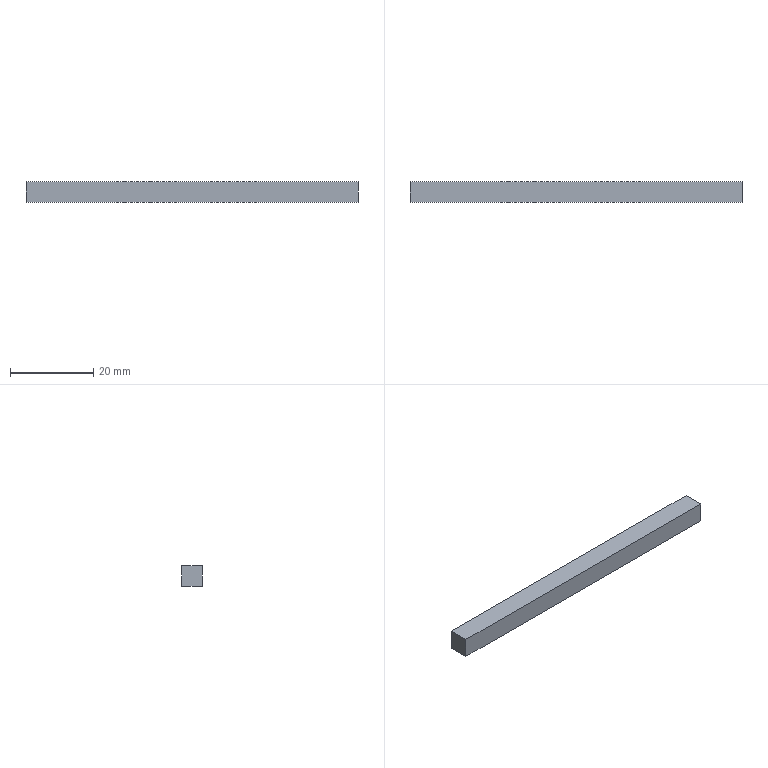Part | SolidWorks | features Extrusion 1 | 1 solid | 6 faces | box 80 x 5 x 5 mm | volume 2000 mm3 | plane 6
STEP:
#1=CARTESIAN_POINT('',(0.,5.,0.));
#2=VERTEX_POINT('',#1);
#3=CARTESIAN_POINT('',(0.,0.,0.));
#4=VERTEX_POINT('',#3);
#5=CARTESIAN_POINT('',(0.,0.,0.));
#6=DIRECTION('',(0.,-1.,0.));
#7=VECTOR('',#6,1000.);
#8=LINE('',#5,#7);
#9=EDGE_CURVE('',#2,#4,#8,.T.);
#10=ORIENTED_EDGE('',*,*,#9,.T.);
#11=CARTESIAN_POINT('',(0.,0.,5.));
#12=VERTEX_POINT('',#11);
#13=CARTESIAN_POINT('',(0.,0.,5.));
#14=DIRECTION('',(0.,0.,-1.));
#15=VECTOR('',#14,1000.);
#16=LINE('',#13,#15);
#17=EDGE_CURVE('',#12,#4,#16,.T.);
#18=ORIENTED_EDGE('',*,*,#17,.F.);
#19=CARTESIAN_POINT('',(0.,5.,5.));
#20=VERTEX_POINT('',#19);
#21=CARTESIAN_POINT('',(0.,0.,5.));
#22=DIRECTION('',(0.,-1.,0.));
#23=VECTOR('',#22,1000.);
#24=LINE('',#21,#23);
#25=EDGE_CURVE('',#20,#12,#24,.T.);
#26=ORIENTED_EDGE('',*,*,#25,.F.);
#27=CARTESIAN_POINT('',(0.,5.,5.));
#28=DIRECTION('',(0.,0.,-1.));
#29=VECTOR('',#28,1000.);
#30=LINE('',#27,#29);
#31=EDGE_CURVE('',#20,#2,#30,.T.);
#32=ORIENTED_EDGE('',*,*,#31,.T.);
#33=EDGE_LOOP('',(#10,#18,#26,#32));
#34=FACE_OUTER_BOUND('',#33,.T.);
#35=CARTESIAN_POINT('',(0.,0.,5.));
#36=DIRECTION('',(1.,0.,0.));
#37=DIRECTION('',(0.,0.,-1.));
#38=AXIS2_PLACEMENT_3D('',#35,#36,#37);
#39=PLANE('',#38);
#40=ADVANCED_FACE('',(#34),#39,.F.);
#41=CARTESIAN_POINT('',(80.,0.,0.));
#42=VERTEX_POINT('',#41);
#43=CARTESIAN_POINT('',(0.,0.,0.));
#44=DIRECTION('',(1.,0.,0.));
#45=VECTOR('',#44,1000.);
#46=LINE('',#43,#45);
#47=EDGE_CURVE('',#4,#42,#46,.T.);
#48=ORIENTED_EDGE('',*,*,#47,.T.);
#49=CARTESIAN_POINT('',(80.,0.,5.));
#50=VERTEX_POINT('',#49);
#51=CARTESIAN_POINT('',(80.,0.,5.));
#52=DIRECTION('',(0.,0.,-1.));
#53=VECTOR('',#52,1000.);
#54=LINE('',#51,#53);
#55=EDGE_CURVE('',#50,#42,#54,.T.);
#56=ORIENTED_EDGE('',*,*,#55,.F.);
#57=CARTESIAN_POINT('',(0.,0.,5.));
#58=DIRECTION('',(1.,0.,0.));
#59=VECTOR('',#58,1000.);
#60=LINE('',#57,#59);
#61=EDGE_CURVE('',#12,#50,#60,.T.);
#62=ORIENTED_EDGE('',*,*,#61,.F.);
#63=ORIENTED_EDGE('',*,*,#17,.T.);
#64=EDGE_LOOP('',(#48,#56,#62,#63));
#65=FACE_OUTER_BOUND('',#64,.T.);
#66=CARTESIAN_POINT('',(0.,0.,5.));
#67=DIRECTION('',(0.,1.,0.));
#68=DIRECTION('',(0.,0.,1.));
#69=AXIS2_PLACEMENT_3D('',#66,#67,#68);
#70=PLANE('',#69);
#71=ADVANCED_FACE('',(#65),#70,.F.);
#72=CARTESIAN_POINT('',(80.,5.,0.));
#73=VERTEX_POINT('',#72);
#74=CARTESIAN_POINT('',(80.,0.,0.));
#75=DIRECTION('',(0.,1.,0.));
#76=VECTOR('',#75,1000.);
#77=LINE('',#74,#76);
#78=EDGE_CURVE('',#42,#73,#77,.T.);
#79=ORIENTED_EDGE('',*,*,#78,.T.);
#80=CARTESIAN_POINT('',(80.,5.,5.));
#81=VERTEX_POINT('',#80);
#82=CARTESIAN_POINT('',(80.,5.,5.));
#83=DIRECTION('',(0.,0.,-1.));
#84=VECTOR('',#83,1000.);
#85=LINE('',#82,#84);
#86=EDGE_CURVE('',#81,#73,#85,.T.);
#87=ORIENTED_EDGE('',*,*,#86,.F.);
#88=CARTESIAN_POINT('',(80.,0.,5.));
#89=DIRECTION('',(0.,1.,0.));
#90=VECTOR('',#89,1000.);
#91=LINE('',#88,#90);
#92=EDGE_CURVE('',#50,#81,#91,.T.);
#93=ORIENTED_EDGE('',*,*,#92,.F.);
#94=ORIENTED_EDGE('',*,*,#55,.T.);
#95=EDGE_LOOP('',(#79,#87,#93,#94));
#96=FACE_OUTER_BOUND('',#95,.T.);
#97=CARTESIAN_POINT('',(80.,0.,5.));
#98=DIRECTION('',(-1.,0.,0.));
#99=DIRECTION('',(0.,0.,1.));
#100=AXIS2_PLACEMENT_3D('',#97,#98,#99);
#101=PLANE('',#100);
#102=ADVANCED_FACE('',(#96),#101,.F.);
#103=CARTESIAN_POINT('',(0.,5.,0.));
#104=DIRECTION('',(-1.,0.,0.));
#105=VECTOR('',#104,1000.);
#106=LINE('',#103,#105);
#107=EDGE_CURVE('',#73,#2,#106,.T.);
#108=ORIENTED_EDGE('',*,*,#107,.T.);
#109=ORIENTED_EDGE('',*,*,#31,.F.);
#110=CARTESIAN_POINT('',(0.,5.,5.));
#111=DIRECTION('',(-1.,0.,0.));
#112=VECTOR('',#111,1000.);
#113=LINE('',#110,#112);
#114=EDGE_CURVE('',#81,#20,#113,.T.);
#115=ORIENTED_EDGE('',*,*,#114,.F.);
#116=ORIENTED_EDGE('',*,*,#86,.T.);
#117=EDGE_LOOP('',(#108,#109,#115,#116));
#118=FACE_OUTER_BOUND('',#117,.T.);
#119=CARTESIAN_POINT('',(0.,5.,5.));
#120=DIRECTION('',(0.,-1.,0.));
#121=DIRECTION('',(0.,0.,-1.));
#122=AXIS2_PLACEMENT_3D('',#119,#120,#121);
#123=PLANE('',#122);
#124=ADVANCED_FACE('',(#118),#123,.F.);
#125=ORIENTED_EDGE('',*,*,#25,.T.);
#126=ORIENTED_EDGE('',*,*,#61,.T.);
#127=ORIENTED_EDGE('',*,*,#92,.T.);
#128=ORIENTED_EDGE('',*,*,#114,.T.);
#129=EDGE_LOOP('',(#125,#126,#127,#128));
#130=FACE_OUTER_BOUND('',#129,.T.);
#131=CARTESIAN_POINT('',(0.,0.,5.));
#132=DIRECTION('',(0.,0.,-1.));
#133=DIRECTION('',(-1.,0.,0.));
#134=AXIS2_PLACEMENT_3D('',#131,#132,#133);
#135=PLANE('',#134);
#136=ADVANCED_FACE('',(#130),#135,.F.);
#137=ORIENTED_EDGE('',*,*,#9,.F.);
#138=ORIENTED_EDGE('',*,*,#107,.F.);
#139=ORIENTED_EDGE('',*,*,#78,.F.);
#140=ORIENTED_EDGE('',*,*,#47,.F.);
#141=EDGE_LOOP('',(#137,#138,#139,#140));
#142=FACE_OUTER_BOUND('',#141,.T.);
#143=CARTESIAN_POINT('',(0.,0.,0.));
#144=DIRECTION('',(0.,0.,-1.));
#145=DIRECTION('',(-1.,0.,0.));
#146=AXIS2_PLACEMENT_3D('',#143,#144,#145);
#147=PLANE('',#146);
#148=ADVANCED_FACE('',(#142),#147,.T.);
#149=CLOSED_SHELL('',(#40,#71,#102,#124,#136,#148));
#150=MANIFOLD_SOLID_BREP('',#149);
#151=CARTESIAN_POINT('',(0.,0.,0.));
#152=DIRECTION('',(0.,0.,1.));
#153=DIRECTION('',(1.,0.,0.));
#154=AXIS2_PLACEMENT_3D('',#151,#152,#153);
#155=(LENGTH_UNIT()NAMED_UNIT(*)SI_UNIT(.MILLI.,.METRE.));
#156=UNCERTAINTY_MEASURE_WITH_UNIT(LENGTH_MEASURE(0.00001),#155,'','');
#157=(NAMED_UNIT(*)PLANE_ANGLE_UNIT()SI_UNIT($,.RADIAN.));
#158=(NAMED_UNIT(*)SI_UNIT($,.STERADIAN.)SOLID_ANGLE_UNIT());
#159=(GEOMETRIC_REPRESENTATION_CONTEXT(3)GLOBAL_UNCERTAINTY_ASSIGNED_CONTEXT((#156))GLOBAL_UNIT_ASSIGNED_CONTEXT((#155,#157,#158))REPRESENTATION_CONTEXT('',''));
#160=ADVANCED_BREP_SHAPE_REPRESENTATION('',(#150,#154),#159);